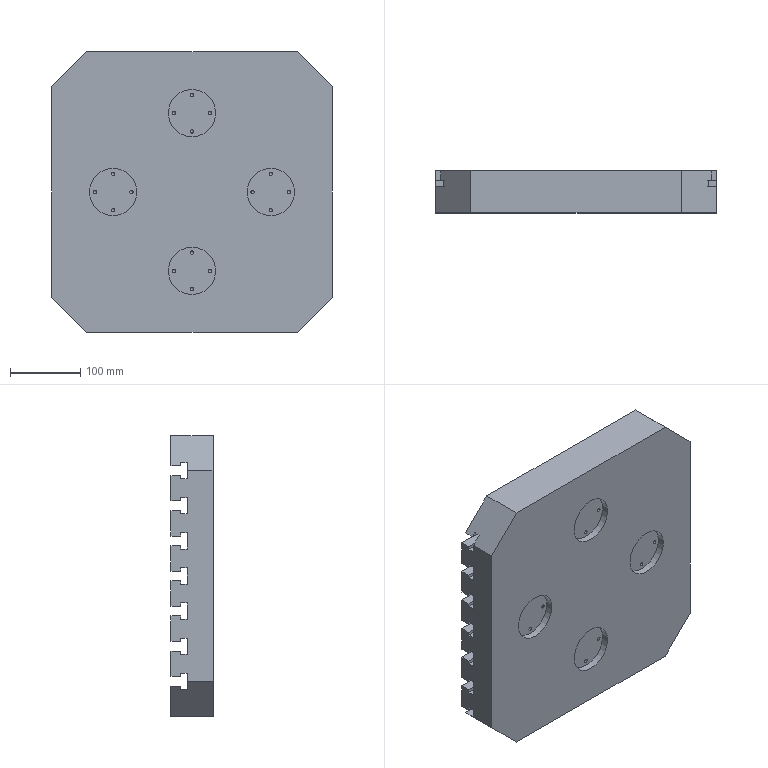Part | STEP file | Satellite table | 1 solid | 106 faces | box 400 x 60 x 400 mm | volume 8025987 mm3 | plane 70 | cylinder 20 | cone 16 | commonest cylinder face diameters 4.917 x16 67.5 x4